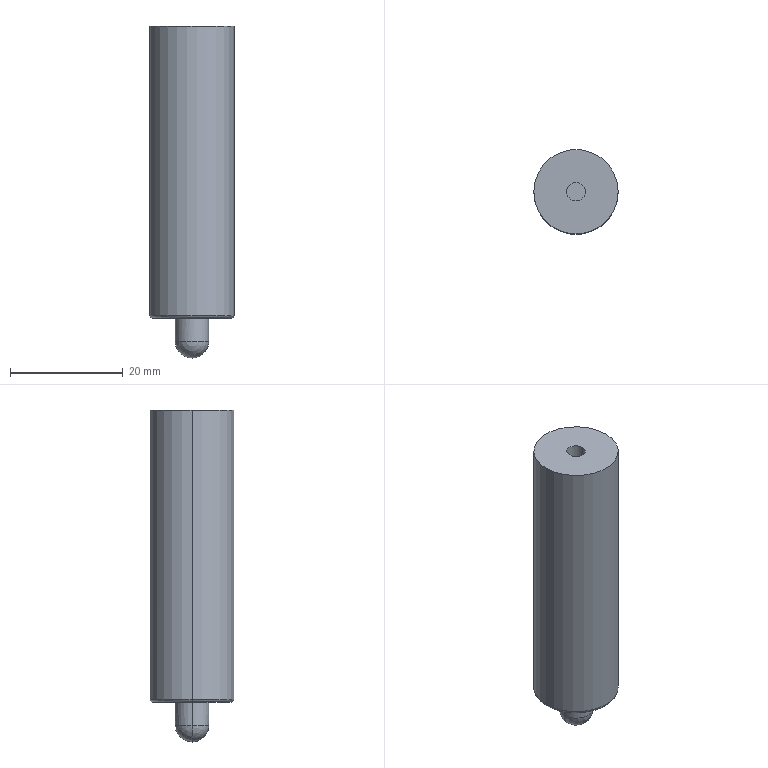Part | SolidWorks | features BaseBody 1 | 1 solid | 14 faces | box 15 x 15 x 59 mm | volume 9171 mm3 | cylinder 6 | torus 3 | plane 3 | sphere 2 | commonest cylinder face diameters 3.3 x2 6 x2 15 x2
STEP:
#1=CARTESIAN_POINT('',(-760.63,615.893,443.08));
#2=VERTEX_POINT('',#1);
#3=CARTESIAN_POINT('',(-775.63,615.797,443.08));
#4=VERTEX_POINT('',#3);
#5=CARTESIAN_POINT('',(-768.13,615.797,443.08));
#6=DIRECTION('',(0.,0.,1.));
#7=DIRECTION('',(0.9999,0.01286,0.));
#8=AXIS2_PLACEMENT_3D('',#5,#6,#7);
#9=CIRCLE('',#8,7.5);
#10=EDGE_CURVE('',#2,#4,#9,.T.);
#11=ORIENTED_EDGE('',*,*,#10,.F.);
#12=CARTESIAN_POINT('',(-761.13,615.887,442.58));
#13=VERTEX_POINT('',#12);
#14=CARTESIAN_POINT('',(-761.13,615.887,443.08));
#15=DIRECTION('',(-0.01286,0.9999,0.));
#16=DIRECTION('',(-0.9999,-0.01286,0.));
#17=AXIS2_PLACEMENT_3D('',#14,#15,#16);
#18=CIRCLE('',#17,0.5);
#19=EDGE_CURVE('',#2,#13,#18,.T.);
#20=ORIENTED_EDGE('',*,*,#19,.T.);
#21=CARTESIAN_POINT('',(-775.13,615.797,442.58));
#22=VERTEX_POINT('',#21);
#23=CARTESIAN_POINT('',(-768.13,615.797,442.58));
#24=DIRECTION('',(0.,0.,1.));
#25=DIRECTION('',(1.,0.000001544,0.));
#26=AXIS2_PLACEMENT_3D('',#23,#24,#25);
#27=CIRCLE('',#26,7.);
#28=EDGE_CURVE('',#13,#22,#27,.T.);
#29=ORIENTED_EDGE('',*,*,#28,.T.);
#30=CARTESIAN_POINT('',(-775.13,615.797,443.08));
#31=DIRECTION('',(0.000001544,-1.,0.));
#32=DIRECTION('',(-1.,-0.000001544,0.));
#33=AXIS2_PLACEMENT_3D('',#30,#31,#32);
#34=CIRCLE('',#33,0.5);
#35=EDGE_CURVE('',#4,#22,#34,.T.);
#36=ORIENTED_EDGE('',*,*,#35,.F.);
#37=EDGE_LOOP('',(#11,#20,#29,#36));
#38=FACE_OUTER_BOUND('',#37,.T.);
#39=CARTESIAN_POINT('',(-768.13,615.797,443.08));
#40=DIRECTION('',(0.,0.,-1.));
#41=DIRECTION('',(0.9999,0.01286,0.));
#42=AXIS2_PLACEMENT_3D('',#39,#40,#41);
#43=TOROIDAL_SURFACE('',#42,7.,0.5);
#44=ADVANCED_FACE('',(#38),#43,.T.);
#45=CARTESIAN_POINT('',(-775.63,615.797,494.482));
#46=VERTEX_POINT('',#45);
#47=CARTESIAN_POINT('',(-760.63,615.797,494.482));
#48=VERTEX_POINT('',#47);
#49=CARTESIAN_POINT('',(-768.13,615.797,494.482));
#50=DIRECTION('',(0.,0.,-1.));
#51=DIRECTION('',(-1.,-0.000001544,0.));
#52=AXIS2_PLACEMENT_3D('',#49,#50,#51);
#53=CIRCLE('',#52,7.5);
#54=EDGE_CURVE('',#46,#48,#53,.T.);
#55=ORIENTED_EDGE('',*,*,#54,.F.);
#56=CARTESIAN_POINT('',(-768.13,615.797,494.482));
#57=DIRECTION('',(0.,0.,-1.));
#58=DIRECTION('',(1.,0.000001544,0.));
#59=AXIS2_PLACEMENT_3D('',#56,#57,#58);
#60=CIRCLE('',#59,7.5);
#61=EDGE_CURVE('',#48,#46,#60,.T.);
#62=ORIENTED_EDGE('',*,*,#61,.F.);
#63=EDGE_LOOP('',(#55,#62));
#64=FACE_OUTER_BOUND('',#63,.T.);
#65=CARTESIAN_POINT('',(-766.48,615.797,494.482));
#66=VERTEX_POINT('',#65);
#67=CARTESIAN_POINT('',(-769.78,615.797,494.482));
#68=VERTEX_POINT('',#67);
#69=CARTESIAN_POINT('',(-768.13,615.797,494.482));
#70=DIRECTION('',(0.,0.,1.));
#71=DIRECTION('',(1.,0.000001544,0.));
#72=AXIS2_PLACEMENT_3D('',#69,#70,#71);
#73=CIRCLE('',#72,1.65);
#74=EDGE_CURVE('',#66,#68,#73,.T.);
#75=ORIENTED_EDGE('',*,*,#74,.F.);
#76=CARTESIAN_POINT('',(-768.13,615.797,494.482));
#77=DIRECTION('',(0.,0.,1.));
#78=DIRECTION('',(-1.,-0.000001544,0.));
#79=AXIS2_PLACEMENT_3D('',#76,#77,#78);
#80=CIRCLE('',#79,1.65);
#81=EDGE_CURVE('',#68,#66,#80,.T.);
#82=ORIENTED_EDGE('',*,*,#81,.F.);
#83=EDGE_LOOP('',(#75,#82));
#84=FACE_BOUND('',#83,.T.);
#85=CARTESIAN_POINT('',(-69.998,0.001241,494.482));
#86=DIRECTION('',(0.,0.,-1.));
#87=DIRECTION('',(1.,0.000001544,0.));
#88=AXIS2_PLACEMENT_3D('',#85,#86,#87);
#89=PLANE('',#88);
#90=ADVANCED_FACE('',(#64,#84),#89,.F.);
#91=ORIENTED_EDGE('',*,*,#61,.T.);
#92=CARTESIAN_POINT('',(-775.63,615.797,494.482));
#93=DIRECTION('',(0.,0.,-1.));
#94=VECTOR('',#93,1000.);
#95=LINE('',#92,#94);
#96=EDGE_CURVE('',#46,#4,#95,.T.);
#97=ORIENTED_EDGE('',*,*,#96,.T.);
#98=CARTESIAN_POINT('',(-760.63,615.797,443.08));
#99=VERTEX_POINT('',#98);
#100=CARTESIAN_POINT('',(-768.13,615.797,443.08));
#101=DIRECTION('',(0.,0.,1.));
#102=DIRECTION('',(-1.,-0.000001544,0.));
#103=AXIS2_PLACEMENT_3D('',#100,#101,#102);
#104=CIRCLE('',#103,7.5);
#105=EDGE_CURVE('',#4,#99,#104,.T.);
#106=ORIENTED_EDGE('',*,*,#105,.T.);
#107=CARTESIAN_POINT('',(-760.63,615.797,443.08));
#108=DIRECTION('',(0.,0.,1.));
#109=VECTOR('',#108,1000.);
#110=LINE('',#107,#109);
#111=EDGE_CURVE('',#99,#48,#110,.T.);
#112=ORIENTED_EDGE('',*,*,#111,.T.);
#113=EDGE_LOOP('',(#91,#97,#106,#112));
#114=FACE_OUTER_BOUND('',#113,.T.);
#115=CARTESIAN_POINT('',(-768.13,615.797,442.58));
#116=DIRECTION('',(0.,0.,-1.));
#117=DIRECTION('',(1.,0.000001544,0.));
#118=AXIS2_PLACEMENT_3D('',#115,#116,#117);
#119=CYLINDRICAL_SURFACE('',#118,7.5);
#120=ADVANCED_FACE('',(#114),#119,.T.);
#121=ORIENTED_EDGE('',*,*,#54,.T.);
#122=ORIENTED_EDGE('',*,*,#111,.F.);
#123=CARTESIAN_POINT('',(-768.13,615.797,443.08));
#124=DIRECTION('',(0.,0.,1.));
#125=DIRECTION('',(0.9999,0.01286,0.));
#126=AXIS2_PLACEMENT_3D('',#123,#124,#125);
#127=CIRCLE('',#126,7.5);
#128=EDGE_CURVE('',#99,#2,#127,.T.);
#129=ORIENTED_EDGE('',*,*,#128,.T.);
#130=ORIENTED_EDGE('',*,*,#10,.T.);
#131=ORIENTED_EDGE('',*,*,#96,.F.);
#132=EDGE_LOOP('',(#121,#122,#129,#130,#131));
#133=FACE_OUTER_BOUND('',#132,.T.);
#134=CARTESIAN_POINT('',(-768.13,615.797,442.58));
#135=DIRECTION('',(0.,0.,-1.));
#136=DIRECTION('',(1.,0.000001544,0.));
#137=AXIS2_PLACEMENT_3D('',#134,#135,#136);
#138=CYLINDRICAL_SURFACE('',#137,7.5);
#139=ADVANCED_FACE('',(#133),#138,.T.);
#140=ORIENTED_EDGE('',*,*,#19,.F.);
#141=ORIENTED_EDGE('',*,*,#128,.F.);
#142=CARTESIAN_POINT('',(-761.13,615.797,442.58));
#143=VERTEX_POINT('',#142);
#144=CARTESIAN_POINT('',(-761.13,615.797,443.08));
#145=DIRECTION('',(0.000001544,-1.,0.));
#146=DIRECTION('',(0.,0.,-1.));
#147=AXIS2_PLACEMENT_3D('',#144,#145,#146);
#148=CIRCLE('',#147,0.5);
#149=EDGE_CURVE('',#143,#99,#148,.T.);
#150=ORIENTED_EDGE('',*,*,#149,.F.);
#151=CARTESIAN_POINT('',(-768.13,615.797,442.58));
#152=DIRECTION('',(0.,0.,1.));
#153=DIRECTION('',(1.,0.000001544,0.));
#154=AXIS2_PLACEMENT_3D('',#151,#152,#153);
#155=CIRCLE('',#154,7.);
#156=EDGE_CURVE('',#143,#13,#155,.T.);
#157=ORIENTED_EDGE('',*,*,#156,.T.);
#158=EDGE_LOOP('',(#140,#141,#150,#157));
#159=FACE_OUTER_BOUND('',#158,.T.);
#160=CARTESIAN_POINT('',(-768.13,615.797,443.08));
#161=DIRECTION('',(0.,0.,-1.));
#162=DIRECTION('',(0.9999,0.01286,0.));
#163=AXIS2_PLACEMENT_3D('',#160,#161,#162);
#164=TOROIDAL_SURFACE('',#163,7.,0.5);
#165=ADVANCED_FACE('',(#159),#164,.T.);
#166=ORIENTED_EDGE('',*,*,#105,.F.);
#167=ORIENTED_EDGE('',*,*,#35,.T.);
#168=CARTESIAN_POINT('',(-768.13,615.797,442.58));
#169=DIRECTION('',(0.,0.,1.));
#170=DIRECTION('',(-1.,-0.000001544,0.));
#171=AXIS2_PLACEMENT_3D('',#168,#169,#170);
#172=CIRCLE('',#171,7.);
#173=EDGE_CURVE('',#22,#143,#172,.T.);
#174=ORIENTED_EDGE('',*,*,#173,.T.);
#175=ORIENTED_EDGE('',*,*,#149,.T.);
#176=EDGE_LOOP('',(#166,#167,#174,#175));
#177=FACE_OUTER_BOUND('',#176,.T.);
#178=CARTESIAN_POINT('',(-768.13,615.797,443.08));
#179=DIRECTION('',(0.,0.,-1.));
#180=DIRECTION('',(1.,0.000001544,0.));
#181=AXIS2_PLACEMENT_3D('',#178,#179,#180);
#182=TOROIDAL_SURFACE('',#181,7.,0.5);
#183=ADVANCED_FACE('',(#177),#182,.T.);
#184=ORIENTED_EDGE('',*,*,#173,.F.);
#185=ORIENTED_EDGE('',*,*,#28,.F.);
#186=ORIENTED_EDGE('',*,*,#156,.F.);
#187=EDGE_LOOP('',(#184,#185,#186));
#188=FACE_OUTER_BOUND('',#187,.T.);
#189=CARTESIAN_POINT('',(-765.13,615.797,442.58));
#190=VERTEX_POINT('',#189);
#191=CARTESIAN_POINT('',(-771.13,615.797,442.58));
#192=VERTEX_POINT('',#191);
#193=CARTESIAN_POINT('',(-768.13,615.797,442.58));
#194=DIRECTION('',(0.,0.,-1.));
#195=DIRECTION('',(1.,0.000001544,0.));
#196=AXIS2_PLACEMENT_3D('',#193,#194,#195);
#197=CIRCLE('',#196,3.);
#198=EDGE_CURVE('',#190,#192,#197,.T.);
#199=ORIENTED_EDGE('',*,*,#198,.F.);
#200=CARTESIAN_POINT('',(-768.13,615.797,442.58));
#201=DIRECTION('',(0.,0.,-1.));
#202=DIRECTION('',(-1.,-0.000001544,0.));
#203=AXIS2_PLACEMENT_3D('',#200,#201,#202);
#204=CIRCLE('',#203,3.);
#205=EDGE_CURVE('',#192,#190,#204,.T.);
#206=ORIENTED_EDGE('',*,*,#205,.F.);
#207=EDGE_LOOP('',(#199,#206));
#208=FACE_BOUND('',#207,.T.);
#209=CARTESIAN_POINT('',(-723.13,626.297,442.58));
#210=DIRECTION('',(0.,0.,1.));
#211=DIRECTION('',(-0.000001544,1.,0.));
#212=AXIS2_PLACEMENT_3D('',#209,#210,#211);
#213=PLANE('',#212);
#214=ADVANCED_FACE('',(#188,#208),#213,.F.);
#215=ORIENTED_EDGE('',*,*,#205,.T.);
#216=CARTESIAN_POINT('',(-765.13,615.797,438.482));
#217=VERTEX_POINT('',#216);
#218=CARTESIAN_POINT('',(-765.13,615.797,442.58));
#219=DIRECTION('',(0.,0.,-1.));
#220=VECTOR('',#219,1000.);
#221=LINE('',#218,#220);
#222=EDGE_CURVE('',#190,#217,#221,.T.);
#223=ORIENTED_EDGE('',*,*,#222,.T.);
#224=CARTESIAN_POINT('',(-771.13,615.797,438.482));
#225=VERTEX_POINT('',#224);
#226=CARTESIAN_POINT('',(-768.13,615.797,438.482));
#227=DIRECTION('',(0.,0.,1.));
#228=DIRECTION('',(1.,0.000001544,0.));
#229=AXIS2_PLACEMENT_3D('',#226,#227,#228);
#230=CIRCLE('',#229,3.);
#231=EDGE_CURVE('',#217,#225,#230,.T.);
#232=ORIENTED_EDGE('',*,*,#231,.T.);
#233=CARTESIAN_POINT('',(-771.13,615.797,438.482));
#234=DIRECTION('',(0.,0.,1.));
#235=VECTOR('',#234,1000.);
#236=LINE('',#233,#235);
#237=EDGE_CURVE('',#225,#192,#236,.T.);
#238=ORIENTED_EDGE('',*,*,#237,.T.);
#239=EDGE_LOOP('',(#215,#223,#232,#238));
#240=FACE_OUTER_BOUND('',#239,.T.);
#241=CARTESIAN_POINT('',(-768.13,615.797,442.58));
#242=DIRECTION('',(0.,0.,-1.));
#243=DIRECTION('',(1.,0.000001544,0.));
#244=AXIS2_PLACEMENT_3D('',#241,#242,#243);
#245=CYLINDRICAL_SURFACE('',#244,3.);
#246=ADVANCED_FACE('',(#240),#245,.T.);
#247=ORIENTED_EDGE('',*,*,#198,.T.);
#248=ORIENTED_EDGE('',*,*,#237,.F.);
#249=CARTESIAN_POINT('',(-768.13,615.797,438.482));
#250=DIRECTION('',(0.,0.,1.));
#251=DIRECTION('',(-1.,-0.000001544,0.));
#252=AXIS2_PLACEMENT_3D('',#249,#250,#251);
#253=CIRCLE('',#252,3.);
#254=EDGE_CURVE('',#225,#217,#253,.T.);
#255=ORIENTED_EDGE('',*,*,#254,.T.);
#256=ORIENTED_EDGE('',*,*,#222,.F.);
#257=EDGE_LOOP('',(#247,#248,#255,#256));
#258=FACE_OUTER_BOUND('',#257,.T.);
#259=CARTESIAN_POINT('',(-768.13,615.797,442.58));
#260=DIRECTION('',(0.,0.,-1.));
#261=DIRECTION('',(1.,0.000001544,0.));
#262=AXIS2_PLACEMENT_3D('',#259,#260,#261);
#263=CYLINDRICAL_SURFACE('',#262,3.);
#264=ADVANCED_FACE('',(#258),#263,.T.);
#265=CARTESIAN_POINT('',(-768.13,615.797,435.482));
#266=VERTEX_POINT('',#265);
#267=CARTESIAN_POINT('',(-768.13,615.797,438.482));
#268=DIRECTION('',(-0.000001545,1.,0.));
#269=DIRECTION('',(1.,0.000001545,0.));
#270=AXIS2_PLACEMENT_3D('',#267,#268,#269);
#271=CIRCLE('',#270,3.);
#272=EDGE_CURVE('',#217,#266,#271,.T.);
#273=ORIENTED_EDGE('',*,*,#272,.F.);
#274=ORIENTED_EDGE('',*,*,#254,.F.);
#275=CARTESIAN_POINT('',(-768.13,615.797,438.482));
#276=DIRECTION('',(-0.000001544,1.,0.));
#277=DIRECTION('',(0.,0.,-1.));
#278=AXIS2_PLACEMENT_3D('',#275,#276,#277);
#279=CIRCLE('',#278,3.);
#280=EDGE_CURVE('',#266,#225,#279,.T.);
#281=ORIENTED_EDGE('',*,*,#280,.F.);
#282=EDGE_LOOP('',(#273,#274,#281));
#283=FACE_OUTER_BOUND('',#282,.T.);
#284=CARTESIAN_POINT('',(-768.13,615.797,438.482));
#285=DIRECTION('',(0.000001544,-1.,0.));
#286=DIRECTION('',(1.,0.000001544,0.));
#287=AXIS2_PLACEMENT_3D('',#284,#285,#286);
#288=SPHERICAL_SURFACE('',#287,3.);
#289=ADVANCED_FACE('',(#283),#288,.T.);
#290=ORIENTED_EDGE('',*,*,#280,.T.);
#291=ORIENTED_EDGE('',*,*,#231,.F.);
#292=ORIENTED_EDGE('',*,*,#272,.T.);
#293=EDGE_LOOP('',(#290,#291,#292));
#294=FACE_OUTER_BOUND('',#293,.T.);
#295=CARTESIAN_POINT('',(-768.13,615.797,438.482));
#296=DIRECTION('',(0.000001544,-1.,0.));
#297=DIRECTION('',(1.,0.000001544,0.));
#298=AXIS2_PLACEMENT_3D('',#295,#296,#297);
#299=SPHERICAL_SURFACE('',#298,3.);
#300=ADVANCED_FACE('',(#294),#299,.T.);
#301=CARTESIAN_POINT('',(-766.48,615.797,474.482));
#302=VERTEX_POINT('',#301);
#303=CARTESIAN_POINT('',(-769.78,615.797,474.482));
#304=VERTEX_POINT('',#303);
#305=CARTESIAN_POINT('',(-768.13,615.797,474.482));
#306=DIRECTION('',(0.,0.,-1.));
#307=DIRECTION('',(1.,0.000001544,0.));
#308=AXIS2_PLACEMENT_3D('',#305,#306,#307);
#309=CIRCLE('',#308,1.65);
#310=EDGE_CURVE('',#302,#304,#309,.T.);
#311=ORIENTED_EDGE('',*,*,#310,.T.);
#312=CARTESIAN_POINT('',(-769.78,615.797,474.482));
#313=DIRECTION('',(0.,0.,1.));
#314=VECTOR('',#313,1000.);
#315=LINE('',#312,#314);
#316=EDGE_CURVE('',#304,#68,#315,.T.);
#317=ORIENTED_EDGE('',*,*,#316,.T.);
#318=ORIENTED_EDGE('',*,*,#81,.T.);
#319=CARTESIAN_POINT('',(-766.48,615.797,494.482));
#320=DIRECTION('',(0.,0.,-1.));
#321=VECTOR('',#320,1000.);
#322=LINE('',#319,#321);
#323=EDGE_CURVE('',#66,#302,#322,.T.);
#324=ORIENTED_EDGE('',*,*,#323,.T.);
#325=EDGE_LOOP('',(#311,#317,#318,#324));
#326=FACE_OUTER_BOUND('',#325,.T.);
#327=CARTESIAN_POINT('',(-768.13,615.797,494.482));
#328=DIRECTION('',(0.,0.,1.));
#329=DIRECTION('',(-1.,-0.000001544,0.));
#330=AXIS2_PLACEMENT_3D('',#327,#328,#329);
#331=CYLINDRICAL_SURFACE('',#330,1.65);
#332=ADVANCED_FACE('',(#326),#331,.F.);
#333=CARTESIAN_POINT('',(-768.13,615.797,474.482));
#334=DIRECTION('',(0.,0.,-1.));
#335=DIRECTION('',(-1.,-0.000001544,0.));
#336=AXIS2_PLACEMENT_3D('',#333,#334,#335);
#337=CIRCLE('',#336,1.65);
#338=EDGE_CURVE('',#304,#302,#337,.T.);
#339=ORIENTED_EDGE('',*,*,#338,.T.);
#340=ORIENTED_EDGE('',*,*,#323,.F.);
#341=ORIENTED_EDGE('',*,*,#74,.T.);
#342=ORIENTED_EDGE('',*,*,#316,.F.);
#343=EDGE_LOOP('',(#339,#340,#341,#342));
#344=FACE_OUTER_BOUND('',#343,.T.);
#345=CARTESIAN_POINT('',(-768.13,615.797,494.482));
#346=DIRECTION('',(0.,0.,1.));
#347=DIRECTION('',(-1.,-0.000001544,0.));
#348=AXIS2_PLACEMENT_3D('',#345,#346,#347);
#349=CYLINDRICAL_SURFACE('',#348,1.65);
#350=ADVANCED_FACE('',(#344),#349,.F.);
#351=ORIENTED_EDGE('',*,*,#338,.F.);
#352=ORIENTED_EDGE('',*,*,#310,.F.);
#353=EDGE_LOOP('',(#351,#352));
#354=FACE_OUTER_BOUND('',#353,.T.);
#355=CARTESIAN_POINT('',(-69.998,0.001241,474.482));
#356=DIRECTION('',(0.,0.,1.));
#357=DIRECTION('',(-1.,-0.000001544,0.));
#358=AXIS2_PLACEMENT_3D('',#355,#356,#357);
#359=PLANE('',#358);
#360=ADVANCED_FACE('',(#354),#359,.T.);
#361=CLOSED_SHELL('',(#44,#90,#120,#139,#165,#183,#214,#246,#264,#289,#300,#332,#350,#360));
#362=MANIFOLD_SOLID_BREP('',#361);
#363=CARTESIAN_POINT('',(0.,0.,0.));
#364=DIRECTION('',(0.,0.,1.));
#365=DIRECTION('',(1.,0.,0.));
#366=AXIS2_PLACEMENT_3D('',#363,#364,#365);
#367=(LENGTH_UNIT()NAMED_UNIT(*)SI_UNIT(.MILLI.,.METRE.));
#368=UNCERTAINTY_MEASURE_WITH_UNIT(LENGTH_MEASURE(0.00001),#367,'','');
#369=(NAMED_UNIT(*)PLANE_ANGLE_UNIT()SI_UNIT($,.RADIAN.));
#370=(NAMED_UNIT(*)SI_UNIT($,.STERADIAN.)SOLID_ANGLE_UNIT());
#371=(GEOMETRIC_REPRESENTATION_CONTEXT(3)GLOBAL_UNCERTAINTY_ASSIGNED_CONTEXT((#368))GLOBAL_UNIT_ASSIGNED_CONTEXT((#367,#369,#370))REPRESENTATION_CONTEXT('',''));
#372=ADVANCED_BREP_SHAPE_REPRESENTATION('',(#362,#366),#371);